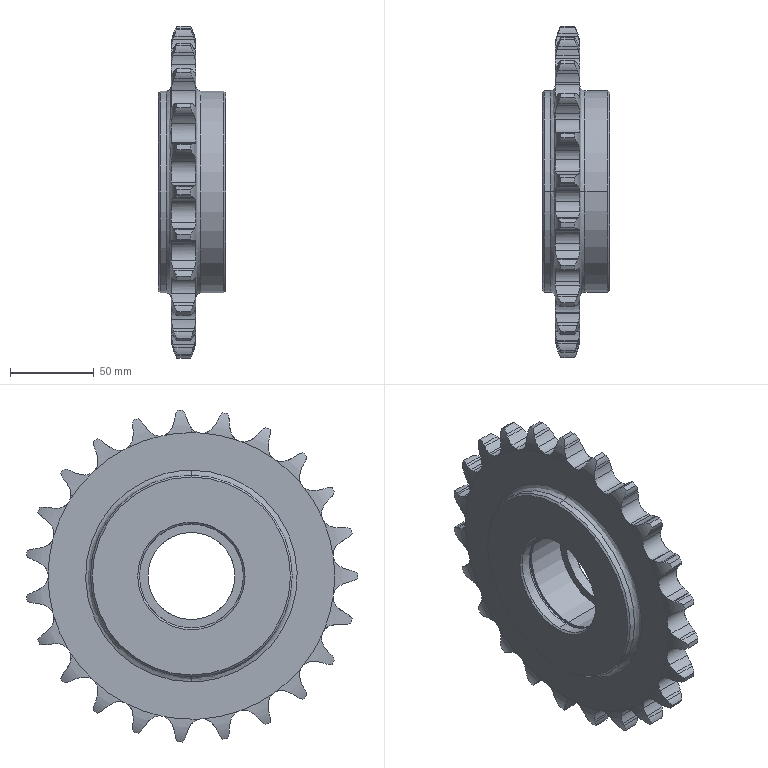Part | STEP file | 1 solid | 275 faces | box 40 x 197.271 x 197.721 mm | volume 545716 mm3 | cylinder 162 | plane 53 | spline 52 | cone 8 | commonest cylinder face diameters 23.032 x49 41.467 x48 16.059 x30 198 x23 62 x4 120 x4